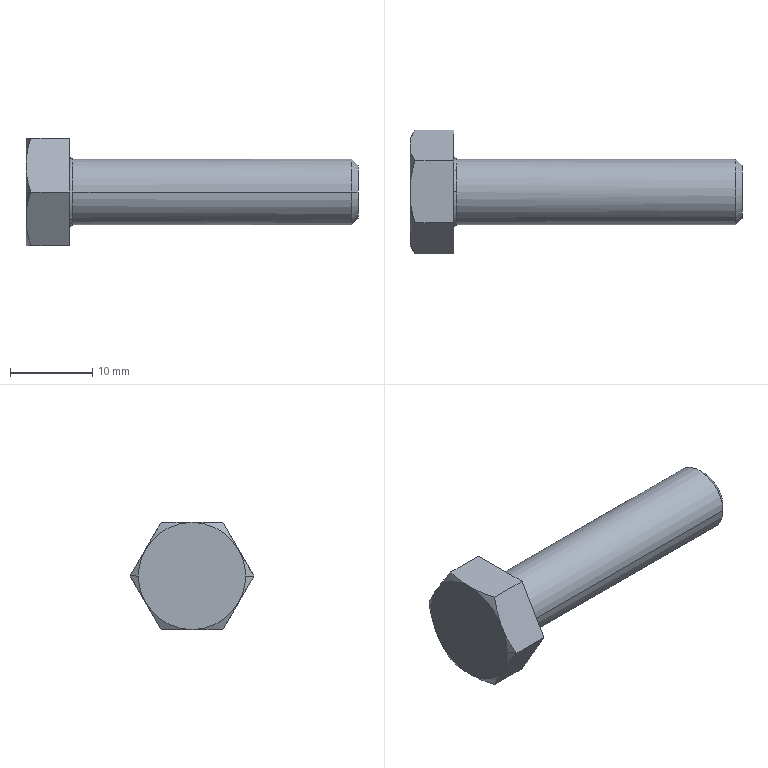Part | STEP file | KS B 1002 - C  M 8 x 35 | 1 solid | 23 faces | box 40.3 x 15.011 x 13 mm | volume 2527 mm3 | cone 10 | plane 9 | torus 2 | cylinder 2 | commonest cylinder face diameters 8 x2